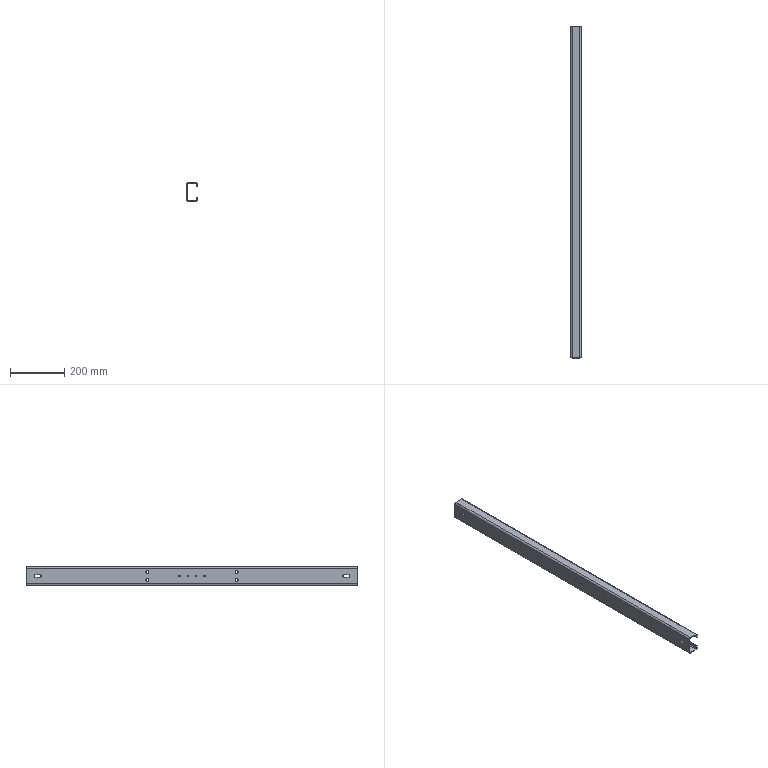Part | SolidWorks | features FlatPattern 1, ICE 1, SMBaseFlange 1, SheetMetal 1 | 1 solid | 62 faces | box 40 x 1228 x 70 mm | volume 399285 mm3 | plane 34 | cylinder 28 | commonest cylinder face diameters 11 x12 7 x8 8 x4 12 x4